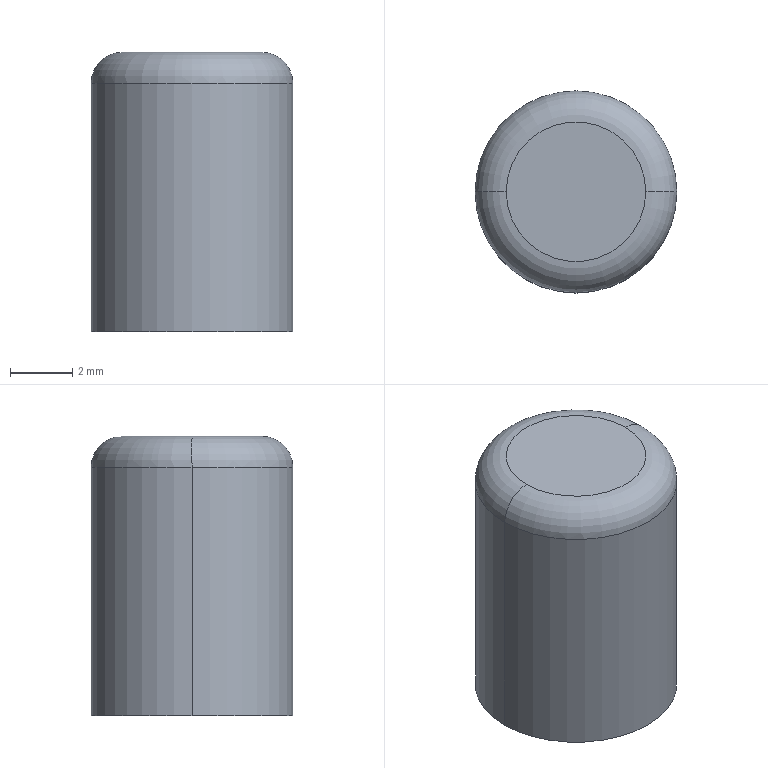Part | STEP file | Pin | 1 solid | 10 faces | box 6.5 x 6.5 x 9 mm | volume 259.622 mm3 | cylinder 4 | cone 2 | torus 2 | plane 2 | commonest cylinder face diameters 2.9 x2 6.5 x2
STEP:
#1=CARTESIAN_POINT('',(1.45,0.,5.));
#2=VERTEX_POINT('',#1);
#3=CARTESIAN_POINT('',(-1.45,0.,5.));
#4=VERTEX_POINT('',#3);
#5=CARTESIAN_POINT('',(0.,0.,5.));
#6=DIRECTION('',(0.,0.,-1.));
#7=DIRECTION('',(-1.,0.,0.));
#8=AXIS2_PLACEMENT_3D('',#5,#6,#7);
#9=CIRCLE('',#8,1.45);
#10=EDGE_CURVE('',#2,#4,#9,.T.);
#11=ORIENTED_EDGE('',*,*,#10,.F.);
#12=CARTESIAN_POINT('',(1.45,0.,0.));
#13=VERTEX_POINT('',#12);
#14=CARTESIAN_POINT('',(1.45,0.,0.));
#15=DIRECTION('',(0.,0.,-1.));
#16=VECTOR('',#15,1000.);
#17=LINE('',#14,#16);
#18=EDGE_CURVE('',#2,#13,#17,.T.);
#19=ORIENTED_EDGE('',*,*,#18,.T.);
#20=CARTESIAN_POINT('',(-1.45,0.,0.));
#21=VERTEX_POINT('',#20);
#22=CARTESIAN_POINT('',(0.,0.,0.));
#23=DIRECTION('',(0.,0.,-1.));
#24=DIRECTION('',(-1.,0.,0.));
#25=AXIS2_PLACEMENT_3D('',#22,#23,#24);
#26=CIRCLE('',#25,1.45);
#27=EDGE_CURVE('',#13,#21,#26,.T.);
#28=ORIENTED_EDGE('',*,*,#27,.T.);
#29=CARTESIAN_POINT('',(-1.45,0.,0.));
#30=DIRECTION('',(0.,0.,-1.));
#31=VECTOR('',#30,1000.);
#32=LINE('',#29,#31);
#33=EDGE_CURVE('',#4,#21,#32,.T.);
#34=ORIENTED_EDGE('',*,*,#33,.F.);
#35=EDGE_LOOP('',(#11,#19,#28,#34));
#36=FACE_OUTER_BOUND('',#35,.T.);
#37=CARTESIAN_POINT('',(0.,0.,0.));
#38=DIRECTION('',(0.,0.,-1.));
#39=DIRECTION('',(-1.,0.,0.));
#40=AXIS2_PLACEMENT_3D('',#37,#38,#39);
#41=CYLINDRICAL_SURFACE('',#40,1.45);
#42=ADVANCED_FACE('',(#36),#41,.F.);
#43=CARTESIAN_POINT('',(0.,0.,5.871));
#44=VERTEX_POINT('',#43);
#45=CARTESIAN_POINT('',(-1.45,0.,5.));
#46=DIRECTION('',(-0.8572,0.,-0.515));
#47=VECTOR('',#46,1000.);
#48=LINE('',#45,#47);
#49=EDGE_CURVE('',#44,#4,#48,.T.);
#50=ORIENTED_EDGE('',*,*,#49,.F.);
#51=CARTESIAN_POINT('',(1.45,0.,5.));
#52=DIRECTION('',(0.8572,0.,-0.515));
#53=VECTOR('',#52,1000.);
#54=LINE('',#51,#53);
#55=EDGE_CURVE('',#44,#2,#54,.T.);
#56=ORIENTED_EDGE('',*,*,#55,.T.);
#57=ORIENTED_EDGE('',*,*,#10,.T.);
#58=EDGE_LOOP('',(#50,#56,#57));
#59=FACE_OUTER_BOUND('',#58,.T.);
#60=CARTESIAN_POINT('',(0.,0.,5.));
#61=DIRECTION('',(0.,0.,-1.));
#62=DIRECTION('',(-1.,0.,0.));
#63=AXIS2_PLACEMENT_3D('',#60,#61,#62);
#64=CONICAL_SURFACE('',#63,1.45,1.03);
#65=ADVANCED_FACE('',(#59),#64,.F.);
#66=CARTESIAN_POINT('',(-3.25,0.,8.));
#67=VERTEX_POINT('',#66);
#68=CARTESIAN_POINT('',(3.25,0.,8.));
#69=VERTEX_POINT('',#68);
#70=CARTESIAN_POINT('',(0.,0.,8.));
#71=DIRECTION('',(0.,0.,-1.));
#72=DIRECTION('',(1.,0.,0.));
#73=AXIS2_PLACEMENT_3D('',#70,#71,#72);
#74=CIRCLE('',#73,3.25);
#75=EDGE_CURVE('',#67,#69,#74,.T.);
#76=ORIENTED_EDGE('',*,*,#75,.F.);
#77=CARTESIAN_POINT('',(-2.25,0.,9.));
#78=VERTEX_POINT('',#77);
#79=CARTESIAN_POINT('',(-2.25,0.,8.));
#80=DIRECTION('',(0.,1.,0.));
#81=DIRECTION('',(-1.,0.,0.));
#82=AXIS2_PLACEMENT_3D('',#79,#80,#81);
#83=CIRCLE('',#82,1.);
#84=EDGE_CURVE('',#67,#78,#83,.T.);
#85=ORIENTED_EDGE('',*,*,#84,.T.);
#86=CARTESIAN_POINT('',(2.25,0.,9.));
#87=VERTEX_POINT('',#86);
#88=CARTESIAN_POINT('',(0.,0.,9.));
#89=DIRECTION('',(0.,0.,1.));
#90=DIRECTION('',(1.,0.,0.));
#91=AXIS2_PLACEMENT_3D('',#88,#89,#90);
#92=CIRCLE('',#91,2.25);
#93=EDGE_CURVE('',#87,#78,#92,.T.);
#94=ORIENTED_EDGE('',*,*,#93,.F.);
#95=CARTESIAN_POINT('',(2.25,0.,8.));
#96=DIRECTION('',(0.,-1.,0.));
#97=DIRECTION('',(0.,0.,-1.));
#98=AXIS2_PLACEMENT_3D('',#95,#96,#97);
#99=CIRCLE('',#98,1.);
#100=EDGE_CURVE('',#69,#87,#99,.T.);
#101=ORIENTED_EDGE('',*,*,#100,.F.);
#102=EDGE_LOOP('',(#76,#85,#94,#101));
#103=FACE_OUTER_BOUND('',#102,.T.);
#104=CARTESIAN_POINT('',(0.,0.,8.));
#105=DIRECTION('',(0.,0.,1.));
#106=DIRECTION('',(1.,0.,0.));
#107=AXIS2_PLACEMENT_3D('',#104,#105,#106);
#108=TOROIDAL_SURFACE('',#107,2.25,1.);
#109=ADVANCED_FACE('',(#103),#108,.T.);
#110=ORIENTED_EDGE('',*,*,#75,.T.);
#111=CARTESIAN_POINT('',(3.25,0.,0.));
#112=VERTEX_POINT('',#111);
#113=CARTESIAN_POINT('',(3.25,0.,9.));
#114=DIRECTION('',(0.,0.,-1.));
#115=VECTOR('',#114,1000.);
#116=LINE('',#113,#115);
#117=EDGE_CURVE('',#69,#112,#116,.T.);
#118=ORIENTED_EDGE('',*,*,#117,.T.);
#119=CARTESIAN_POINT('',(-3.25,0.,0.));
#120=VERTEX_POINT('',#119);
#121=CARTESIAN_POINT('',(0.,0.,0.));
#122=DIRECTION('',(0.,0.,1.));
#123=DIRECTION('',(1.,0.,0.));
#124=AXIS2_PLACEMENT_3D('',#121,#122,#123);
#125=CIRCLE('',#124,3.25);
#126=EDGE_CURVE('',#112,#120,#125,.T.);
#127=ORIENTED_EDGE('',*,*,#126,.T.);
#128=CARTESIAN_POINT('',(-3.25,0.,9.));
#129=DIRECTION('',(0.,0.,-1.));
#130=VECTOR('',#129,1000.);
#131=LINE('',#128,#130);
#132=EDGE_CURVE('',#67,#120,#131,.T.);
#133=ORIENTED_EDGE('',*,*,#132,.F.);
#134=EDGE_LOOP('',(#110,#118,#127,#133));
#135=FACE_OUTER_BOUND('',#134,.T.);
#136=CARTESIAN_POINT('',(0.,0.,9.));
#137=DIRECTION('',(0.,0.,-1.));
#138=DIRECTION('',(-1.,0.,0.));
#139=AXIS2_PLACEMENT_3D('',#136,#137,#138);
#140=CYLINDRICAL_SURFACE('',#139,3.25);
#141=ADVANCED_FACE('',(#135),#140,.T.);
#142=ORIENTED_EDGE('',*,*,#117,.F.);
#143=CARTESIAN_POINT('',(0.,0.,8.));
#144=DIRECTION('',(0.,0.,-1.));
#145=DIRECTION('',(1.,0.,0.));
#146=AXIS2_PLACEMENT_3D('',#143,#144,#145);
#147=CIRCLE('',#146,3.25);
#148=EDGE_CURVE('',#69,#67,#147,.T.);
#149=ORIENTED_EDGE('',*,*,#148,.T.);
#150=ORIENTED_EDGE('',*,*,#132,.T.);
#151=CARTESIAN_POINT('',(0.,0.,0.));
#152=DIRECTION('',(0.,0.,1.));
#153=DIRECTION('',(1.,0.,0.));
#154=AXIS2_PLACEMENT_3D('',#151,#152,#153);
#155=CIRCLE('',#154,3.25);
#156=EDGE_CURVE('',#120,#112,#155,.T.);
#157=ORIENTED_EDGE('',*,*,#156,.T.);
#158=EDGE_LOOP('',(#142,#149,#150,#157));
#159=FACE_OUTER_BOUND('',#158,.T.);
#160=CARTESIAN_POINT('',(0.,0.,9.));
#161=DIRECTION('',(0.,0.,-1.));
#162=DIRECTION('',(-1.,0.,0.));
#163=AXIS2_PLACEMENT_3D('',#160,#161,#162);
#164=CYLINDRICAL_SURFACE('',#163,3.25);
#165=ADVANCED_FACE('',(#159),#164,.T.);
#166=ORIENTED_EDGE('',*,*,#93,.T.);
#167=CARTESIAN_POINT('',(0.,0.,9.));
#168=DIRECTION('',(0.,0.,1.));
#169=DIRECTION('',(1.,0.,0.));
#170=AXIS2_PLACEMENT_3D('',#167,#168,#169);
#171=CIRCLE('',#170,2.25);
#172=EDGE_CURVE('',#78,#87,#171,.T.);
#173=ORIENTED_EDGE('',*,*,#172,.T.);
#174=EDGE_LOOP('',(#166,#173));
#175=FACE_OUTER_BOUND('',#174,.T.);
#176=CARTESIAN_POINT('',(0.,0.,9.));
#177=DIRECTION('',(0.,0.,1.));
#178=DIRECTION('',(1.,0.,0.));
#179=AXIS2_PLACEMENT_3D('',#176,#177,#178);
#180=PLANE('',#179);
#181=ADVANCED_FACE('',(#175),#180,.T.);
#182=CARTESIAN_POINT('',(0.,0.,0.));
#183=DIRECTION('',(0.,0.,-1.));
#184=DIRECTION('',(-1.,0.,0.));
#185=AXIS2_PLACEMENT_3D('',#182,#183,#184);
#186=CIRCLE('',#185,1.45);
#187=EDGE_CURVE('',#21,#13,#186,.T.);
#188=ORIENTED_EDGE('',*,*,#187,.F.);
#189=ORIENTED_EDGE('',*,*,#27,.F.);
#190=EDGE_LOOP('',(#188,#189));
#191=FACE_BOUND('',#190,.T.);
#192=ORIENTED_EDGE('',*,*,#156,.F.);
#193=ORIENTED_EDGE('',*,*,#126,.F.);
#194=EDGE_LOOP('',(#192,#193));
#195=FACE_OUTER_BOUND('',#194,.T.);
#196=CARTESIAN_POINT('',(0.,0.,0.));
#197=DIRECTION('',(0.,0.,1.));
#198=DIRECTION('',(1.,0.,0.));
#199=AXIS2_PLACEMENT_3D('',#196,#197,#198);
#200=PLANE('',#199);
#201=ADVANCED_FACE('',(#191,#195),#200,.F.);
#202=ORIENTED_EDGE('',*,*,#84,.F.);
#203=ORIENTED_EDGE('',*,*,#148,.F.);
#204=ORIENTED_EDGE('',*,*,#100,.T.);
#205=ORIENTED_EDGE('',*,*,#172,.F.);
#206=EDGE_LOOP('',(#202,#203,#204,#205));
#207=FACE_OUTER_BOUND('',#206,.T.);
#208=CARTESIAN_POINT('',(0.,0.,8.));
#209=DIRECTION('',(0.,0.,1.));
#210=DIRECTION('',(1.,0.,0.));
#211=AXIS2_PLACEMENT_3D('',#208,#209,#210);
#212=TOROIDAL_SURFACE('',#211,2.25,1.);
#213=ADVANCED_FACE('',(#207),#212,.T.);
#214=ORIENTED_EDGE('',*,*,#55,.F.);
#215=ORIENTED_EDGE('',*,*,#49,.T.);
#216=CARTESIAN_POINT('',(0.,0.,5.));
#217=DIRECTION('',(0.,0.,-1.));
#218=DIRECTION('',(-1.,0.,0.));
#219=AXIS2_PLACEMENT_3D('',#216,#217,#218);
#220=CIRCLE('',#219,1.45);
#221=EDGE_CURVE('',#4,#2,#220,.T.);
#222=ORIENTED_EDGE('',*,*,#221,.T.);
#223=EDGE_LOOP('',(#214,#215,#222));
#224=FACE_OUTER_BOUND('',#223,.T.);
#225=CARTESIAN_POINT('',(0.,0.,5.));
#226=DIRECTION('',(0.,0.,-1.));
#227=DIRECTION('',(-1.,0.,0.));
#228=AXIS2_PLACEMENT_3D('',#225,#226,#227);
#229=CONICAL_SURFACE('',#228,1.45,1.03);
#230=ADVANCED_FACE('',(#224),#229,.F.);
#231=ORIENTED_EDGE('',*,*,#18,.F.);
#232=ORIENTED_EDGE('',*,*,#221,.F.);
#233=ORIENTED_EDGE('',*,*,#33,.T.);
#234=ORIENTED_EDGE('',*,*,#187,.T.);
#235=EDGE_LOOP('',(#231,#232,#233,#234));
#236=FACE_OUTER_BOUND('',#235,.T.);
#237=CARTESIAN_POINT('',(0.,0.,0.));
#238=DIRECTION('',(0.,0.,-1.));
#239=DIRECTION('',(-1.,0.,0.));
#240=AXIS2_PLACEMENT_3D('',#237,#238,#239);
#241=CYLINDRICAL_SURFACE('',#240,1.45);
#242=ADVANCED_FACE('',(#236),#241,.F.);
#243=CLOSED_SHELL('',(#42,#65,#109,#141,#165,#181,#201,#213,#230,#242));
#244=MANIFOLD_SOLID_BREP('',#243);
#245=CARTESIAN_POINT('',(0.,0.,0.));
#246=DIRECTION('',(0.,0.,1.));
#247=DIRECTION('',(1.,0.,0.));
#248=AXIS2_PLACEMENT_3D('',#245,#246,#247);
#249=(LENGTH_UNIT()NAMED_UNIT(*)SI_UNIT(.MILLI.,.METRE.));
#250=UNCERTAINTY_MEASURE_WITH_UNIT(LENGTH_MEASURE(0.00001),#249,'','');
#251=(NAMED_UNIT(*)PLANE_ANGLE_UNIT()SI_UNIT($,.RADIAN.));
#252=(NAMED_UNIT(*)SI_UNIT($,.STERADIAN.)SOLID_ANGLE_UNIT());
#253=(GEOMETRIC_REPRESENTATION_CONTEXT(3)GLOBAL_UNCERTAINTY_ASSIGNED_CONTEXT((#250))GLOBAL_UNIT_ASSIGNED_CONTEXT((#249,#251,#252))REPRESENTATION_CONTEXT('',''));
#254=ADVANCED_BREP_SHAPE_REPRESENTATION('',(#244,#248),#253);